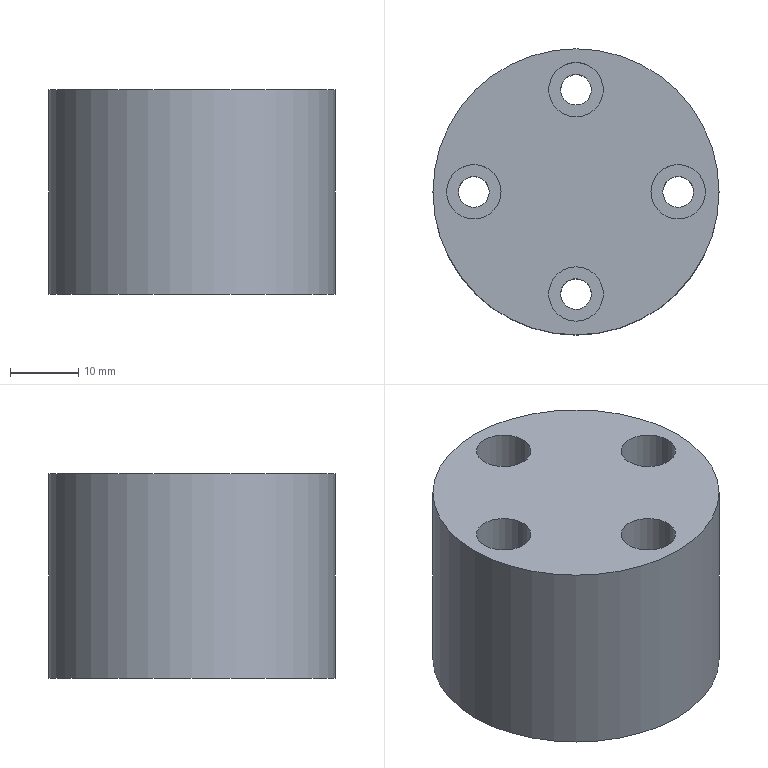NC program | NX | posted with a generic post | part box 42 x 42 x 30 mm
Whole program:
N10 G17 G21 G94 G90
(DRILLING , TOOL : ZXZ)
N12 T01 M6
N14 G54
N16 G17 G0 G90 X0. Y15. S3000 M3
N18 G43 Z30. H1
N20 G94 G81 G98 Z-1. F200. R3.
N22 X-15. Y0.
N24 X0. Y-15.
N26 X15. Y0.
N28 G80
N30 G0 X15. Y0. Z30.
N32 M5
(DRILLING_COPY , TOOL : 4.5ZT)
N34 T02 M6
N36 G54
N38 G17 G0 G90 X0. Y15. S2000 M3
N40 G43 Z30. H2
N42 G94 G83 G98 Z-32.852 F120. Q2. R3.
N44 X-15. Y0.
N46 X0. Y-15.
N48 X15. Y0.
N50 G80
N52 G0 X15. Y0. Z30.
N54 M5
(HOLE_MILLING , TOOL : D6)
N56 T06 M6
N58 G54
N60 G17 G0 G90 X-15. Y0. S4500 M3
N62 G43 Z30. H6
N64 Z0.5
N66 G94 G3 X-14.5 Y-0.5 R0.5 F1400.
N68 X-14. Y0. R0.5
N70 X-14. Y0. Z0.4 I-1. J0.
N72 X-14. Y0. Z0.3 I-1. J0.
N74 X-14. Y0. Z0.2 I-1. J0.
N76 X-14. Y0. Z0.1 I-1. J0.
N78 X-14. Y0. Z0. I-1. J0.
N80 X-14. Y0. Z-0.1 I-1. J0.
N82 X-14. Y0. Z-0.2 I-1. J0.
N84 X-14. Y0. Z-0.3 I-1. J0.
N86 X-14. Y0. Z-0.4 I-1. J0.
N88 X-14. Y0. Z-0.5 I-1. J0.
N90 X-14. Y0. Z-0.6 I-1. J0.
N92 X-14. Y0. Z-0.7 I-1. J0.
N94 X-14. Y0. Z-0.8 I-1. J0.
N96 X-14. Y0. Z-0.9 I-1. J0.
N98 X-14. Y0. Z-1. I-1. J0.
N100 X-14. Y0. Z-1.1 I-1. J0.
N102 X-14. Y0. Z-1.2 I-1. J0.
N104 X-14. Y0. Z-1.3 I-1. J0.
N106 X-14. Y0. Z-1.4 I-1. J0.
N108 X-14. Y0. Z-1.5 I-1. J0.
N110 X-14. Y0. Z-1.6 I-1. J0.
N112 X-14. Y0. Z-1.7 I-1. J0.
N114 X-14. Y0. Z-1.8 I-1. J0.
N116 X-14. Y0. Z-1.9 I-1. J0.
N118 X-14. Y0. Z-2. I-1. J0.
N120 X-14. Y0. Z-2.1 I-1. J0.
N122 X-14. Y0. Z-2.2 I-1. J0.
N124 X-14. Y0. Z-2.3 I-1. J0.
N126 X-14. Y0. Z-2.4 I-1. J0.
N128 X-14. Y0. Z-2.5 I-1. J0.
N130 X-14. Y0. Z-2.6 I-1. J0.
N132 X-14. Y0. Z-2.7 I-1. J0.
N134 X-14. Y0. Z-2.8 I-1. J0.
N136 X-14. Y0. Z-2.9 I-1. J0.
N138 X-14. Y0. Z-3. I-1. J0.
N140 X-14. Y0. Z-3.1 I-1. J0.
N142 X-14. Y0. Z-3.2 I-1. J0.
N144 X-14. Y0. Z-3.3 I-1. J0.
N146 X-14. Y0. Z-3.4 I-1. J0.
N148 X-14. Y0. Z-3.5 I-1. J0.
N150 X-14. Y0. Z-3.6 I-1. J0.
N152 X-14. Y0. Z-3.7 I-1. J0.
N154 X-14. Y0. Z-3.8 I-1. J0.
N156 X-14. Y0. Z-3.9 I-1. J0.
N158 X-14. Y0. Z-4. I-1. J0.
N160 X-14. Y0. Z-4.1 I-1. J0.
N162 X-14. Y0. Z-4.2 I-1. J0.
N164 X-14. Y0. Z-4.3 I-1. J0.
N166 X-14. Y0. Z-4.4 I-1. J0.
N168 X-14. Y0. Z-4.5 I-1. J0.
N170 X-14. Y0. Z-4.6 I-1. J0.
N172 X-14. Y0. Z-4.7 I-1. J0.
N174 X-14. Y0. Z-4.8 I-1. J0.
N176 X-14. Y0. Z-4.9 I-1. J0.
N178 X-14. Y0. Z-5. I-1. J0.
N180 X-14. Y0. Z-5.1 I-1. J0.
N182 X-14. Y0. Z-5.2 I-1. J0.
N184 X-14. Y0. Z-5.3 I-1. J0.
N186 X-14. Y0. Z-5.4 I-1. J0.
N188 X-14. Y0. Z-5.5 I-1. J0.
N190 X-14. Y0. Z-5.6 I-1. J0.
N192 X-14. Y0. Z-5.7 I-1. J0.
N194 X-14. Y0. Z-5.8 I-1. J0.
N196 X-14. Y0. Z-5.9 I-1. J0.
N198 X-14. Y0. Z-6. I-1. J0.
N200 X-15. Y1. R1.
N202 X-14. Y0. R-1.
N204 X-14.5 Y0.5 R0.5
N206 X-15. Y0. R0.5
N208 G0 Z30.
N210 X0. Y15.
N212 Z0.5
N214 G3 X0.5 Y14.5 R0.5
N216 X1. Y15. R0.5
N218 X1. Y15. Z0.4 I-1. J0.
N220 X1. Y15. Z0.3 I-1. J0.
N222 X1. Y15. Z0.2 I-1. J0.
N224 X1. Y15. Z0.1 I-1. J0.
N226 X1. Y15. Z0. I-1. J0.
N228 X1. Y15. Z-0.1 I-1. J0.
N230 X1. Y15. Z-0.2 I-1. J0.
N232 X1. Y15. Z-0.3 I-1. J0.
N234 X1. Y15. Z-0.4 I-1. J0.
N236 X1. Y15. Z-0.5 I-1. J0.
N238 X1. Y15. Z-0.6 I-1. J0.
N240 X1. Y15. Z-0.7 I-1. J0.
N242 X1. Y15. Z-0.8 I-1. J0.
N244 X1. Y15. Z-0.9 I-1. J0.
N246 X1. Y15. Z-1. I-1. J0.
N248 X1. Y15. Z-1.1 I-1. J0.
N250 X1. Y15. Z-1.2 I-1. J0.
N252 X1. Y15. Z-1.3 I-1. J0.
N254 X1. Y15. Z-1.4 I-1. J0.
N256 X1. Y15. Z-1.5 I-1. J0.
N258 X1. Y15. Z-1.6 I-1. J0.
N260 X1. Y15. Z-1.7 I-1. J0.
N262 X1. Y15. Z-1.8 I-1. J0.
N264 X1. Y15. Z-1.9 I-1. J0.
N266 X1. Y15. Z-2. I-1. J0.
N268 X1. Y15. Z-2.1 I-1. J0.
N270 X1. Y15. Z-2.2 I-1. J0.
N272 X1. Y15. Z-2.3 I-1. J0.
N274 X1. Y15. Z-2.4 I-1. J0.
N276 X1. Y15. Z-2.5 I-1. J0.
N278 X1. Y15. Z-2.6 I-1. J0.
N280 X1. Y15. Z-2.7 I-1. J0.
N282 X1. Y15. Z-2.8 I-1. J0.
N284 X1. Y15. Z-2.9 I-1. J0.
N286 X1. Y15. Z-3. I-1. J0.
N288 X1. Y15. Z-3.1 I-1. J0.
N290 X1. Y15. Z-3.2 I-1. J0.
N292 X1. Y15. Z-3.3 I-1. J0.
N294 X1. Y15. Z-3.4 I-1. J0.
N296 X1. Y15. Z-3.5 I-1. J0.
N298 X1. Y15. Z-3.6 I-1. J0.
N300 X1. Y15. Z-3.7 I-1. J0.
N302 X1. Y15. Z-3.8 I-1. J0.
N304 X1. Y15. Z-3.9 I-1. J0.
N306 X1. Y15. Z-4. I-1. J0.
N308 X1. Y15. Z-4.1 I-1. J0.
N310 X1. Y15. Z-4.2 I-1. J0.
N312 X1. Y15. Z-4.3 I-1. J0.
N314 X1. Y15. Z-4.4 I-1. J0.
N316 X1. Y15. Z-4.5 I-1. J0.
N318 X1. Y15. Z-4.6 I-1. J0.
N320 X1. Y15. Z-4.7 I-1. J0.
N322 X1. Y15. Z-4.8 I-1. J0.
N324 X1. Y15. Z-4.9 I-1. J0.
N326 X1. Y15. Z-5. I-1. J0.
N328 X1. Y15. Z-5.1 I-1. J0.
N330 X1. Y15. Z-5.2 I-1. J0.
N332 X1. Y15. Z-5.3 I-1. J0.
N334 X1. Y15. Z-5.4 I-1. J0.
N336 X1. Y15. Z-5.5 I-1. J0.
N338 X1. Y15. Z-5.6 I-1. J0.
N340 X1. Y15. Z-5.7 I-1. J0.
N342 X1. Y15. Z-5.8 I-1. J0.
N344 X1. Y15. Z-5.9 I-1. J0.
N346 X1. Y15. Z-6. I-1. J0.
N348 X0. Y16. R1.
N350 X1. Y15. R-1.
N352 X0.5 Y15.5 R0.5
N354 X0. Y15. R0.5
N356 G0 Z30.
N358 X15. Y0.
N360 Z0.5
N362 G3 X15.5 Y-0.5 R0.5
N364 X16. Y0. R0.5
N366 X16. Y0. Z0.4 I-1. J0.
N368 X16. Y0. Z0.3 I-1. J0.
N370 X16. Y0. Z0.2 I-1. J0.
N372 X16. Y0. Z0.1 I-1. J0.
N374 X16. Y0. Z0. I-1. J0.
N376 X16. Y0. Z-0.1 I-1. J0.
N378 X16. Y0. Z-0.2 I-1. J0.
N380 X16. Y0. Z-0.3 I-1. J0.
N382 X16. Y0. Z-0.4 I-1. J0.
N384 X16. Y0. Z-0.5 I-1. J0.
N386 X16. Y0. Z-0.6 I-1. J0.
N388 X16. Y0. Z-0.7 I-1. J0.
N390 X16. Y0. Z-0.8 I-1. J0.
N392 X16. Y0. Z-0.9 I-1. J0.
N394 X16. Y0. Z-1. I-1. J0.
N396 X16. Y0. Z-1.1 I-1. J0.
N398 X16. Y0. Z-1.2 I-1. J0.
N400 X16. Y0. Z-1.3 I-1. J0.
N402 X16. Y0. Z-1.4 I-1. J0.
N404 X16. Y0. Z-1.5 I-1. J0.
N406 X16. Y0. Z-1.6 I-1. J0.
N408 X16. Y0. Z-1.7 I-1. J0.
N410 X16. Y0. Z-1.8 I-1. J0.
N412 X16. Y0. Z-1.9 I-1. J0.
N414 X16. Y0. Z-2. I-1. J0.
N416 X16. Y0. Z-2.1 I-1. J0.
N418 X16. Y0. Z-2.2 I-1. J0.
N420 X16. Y0. Z-2.3 I-1. J0.
N422 X16. Y0. Z-2.4 I-1. J0.
N424 X16. Y0. Z-2.5 I-1. J0.
N426 X16. Y0. Z-2.6 I-1. J0.
N428 X16. Y0. Z-2.7 I-1. J0.
N430 X16. Y0. Z-2.8 I-1. J0.
N432 X16. Y0. Z-2.9 I-1. J0.
N434 X16. Y0. Z-3. I-1. J0.
N436 X16. Y0. Z-3.1 I-1. J0.
N438 X16. Y0. Z-3.2 I-1. J0.
N440 X16. Y0. Z-3.3 I-1. J0.
N442 X16. Y0. Z-3.4 I-1. J0.
N444 X16. Y0. Z-3.5 I-1. J0.
N446 X16. Y0. Z-3.6 I-1. J0.
N448 X16. Y0. Z-3.7 I-1. J0.
N450 X16. Y0. Z-3.8 I-1. J0.
N452 X16. Y0. Z-3.9 I-1. J0.
N454 X16. Y0. Z-4. I-1. J0.
N456 X16. Y0. Z-4.1 I-1. J0.
N458 X16. Y0. Z-4.2 I-1. J0.
N460 X16. Y0. Z-4.3 I-1. J0.
N462 X16. Y0. Z-4.4 I-1. J0.
N464 X16. Y0. Z-4.5 I-1. J0.
N466 X16. Y0. Z-4.6 I-1. J0.
N468 X16. Y0. Z-4.7 I-1. J0.
N470 X16. Y0. Z-4.8 I-1. J0.
N472 X16. Y0. Z-4.9 I-1. J0.
N474 X16. Y0. Z-5. I-1. J0.
N476 X16. Y0. Z-5.1 I-1. J0.
N478 X16. Y0. Z-5.2 I-1. J0.
N480 X16. Y0. Z-5.3 I-1. J0.
N482 X16. Y0. Z-5.4 I-1. J0.
N484 X16. Y0. Z-5.5 I-1. J0.
N486 X16. Y0. Z-5.6 I-1. J0.
N488 X16. Y0. Z-5.7 I-1. J0.
N490 X16. Y0. Z-5.8 I-1. J0.
N492 X16. Y0. Z-5.9 I-1. J0.
N494 X16. Y0. Z-6. I-1. J0.
N496 X15. Y1. R1.
N498 X16. Y0. R-1.
N500 X15.5 Y0.5 R0.5
N502 X15. Y0. R0.5
N504 G0 Z30.
N506 X0. Y-15.
N508 Z0.5
N510 G3 X0.5 Y-15.5 R0.5
N512 X1. Y-15. R0.5
N514 X1. Y-15. Z0.4 I-1. J0.
N516 X1. Y-15. Z0.3 I-1. J0.
N518 X1. Y-15. Z0.2 I-1. J0.
N520 X1. Y-15. Z0.1 I-1. J0.
N522 X1. Y-15. Z0. I-1. J0.
N524 X1. Y-15. Z-0.1 I-1. J0.
N526 X1. Y-15. Z-0.2 I-1. J0.
N528 X1. Y-15. Z-0.3 I-1. J0.
N530 X1. Y-15. Z-0.4 I-1. J0.
N532 X1. Y-15. Z-0.5 I-1. J0.
N534 X1. Y-15. Z-0.6 I-1. J0.
N536 X1. Y-15. Z-0.7 I-1. J0.
N538 X1. Y-15. Z-0.8 I-1. J0.
N540 X1. Y-15. Z-0.9 I-1. J0.
N542 X1. Y-15. Z-1. I-1. J0.
N544 X1. Y-15. Z-1.1 I-1. J0.
N546 X1. Y-15. Z-1.2 I-1. J0.
N548 X1. Y-15. Z-1.3 I-1. J0.
N550 X1. Y-15. Z-1.4 I-1. J0.
N552 X1. Y-15. Z-1.5 I-1. J0.
N554 X1. Y-15. Z-1.6 I-1. J0.
N556 X1. Y-15. Z-1.7 I-1. J0.
N558 X1. Y-15. Z-1.8 I-1. J0.
N560 X1. Y-15. Z-1.9 I-1. J0.
N562 X1. Y-15. Z-2. I-1. J0.
N564 X1. Y-15. Z-2.1 I-1. J0.
N566 X1. Y-15. Z-2.2 I-1. J0.
N568 X1. Y-15. Z-2.3 I-1. J0.
N570 X1. Y-15. Z-2.4 I-1. J0.
N572 X1. Y-15. Z-2.5 I-1. J0.
N574 X1. Y-15. Z-2.6 I-1. J0.
N576 X1. Y-15. Z-2.7 I-1. J0.
N578 X1. Y-15. Z-2.8 I-1. J0.
N580 X1. Y-15. Z-2.9 I-1. J0.
N582 X1. Y-15. Z-3. I-1. J0.
N584 X1. Y-15. Z-3.1 I-1. J0.
N586 X1. Y-15. Z-3.2 I-1. J0.
N588 X1. Y-15. Z-3.3 I-1. J0.
N590 X1. Y-15. Z-3.4 I-1. J0.
N592 X1. Y-15. Z-3.5 I-1. J0.
N594 X1. Y-15. Z-3.6 I-1. J0.
N596 X1. Y-15. Z-3.7 I-1. J0.
N598 X1. Y-15. Z-3.8 I-1. J0.
N600 X1. Y-15. Z-3.9 I-1. J0.
N602 X1. Y-15. Z-4. I-1. J0.
N604 X1. Y-15. Z-4.1 I-1. J0.
N606 X1. Y-15. Z-4.2 I-1. J0.
N608 X1. Y-15. Z-4.3 I-1. J0.
N610 X1. Y-15. Z-4.4 I-1. J0.
N612 X1. Y-15. Z-4.5 I-1. J0.
N614 X1. Y-15. Z-4.6 I-1. J0.
N616 X1. Y-15. Z-4.7 I-1. J0.
N618 X1. Y-15. Z-4.8 I-1. J0.
N620 X1. Y-15. Z-4.9 I-1. J0.
N622 X1. Y-15. Z-5. I-1. J0.
N624 X1. Y-15. Z-5.1 I-1. J0.
N626 X1. Y-15. Z-5.2 I-1. J0.
N628 X1. Y-15. Z-5.3 I-1. J0.
N630 X1. Y-15. Z-5.4 I-1. J0.
N632 X1. Y-15. Z-5.5 I-1. J0.
N634 X1. Y-15. Z-5.6 I-1. J0.
N636 X1. Y-15. Z-5.7 I-1. J0.
N638 X1. Y-15. Z-5.8 I-1. J0.
N640 X1. Y-15. Z-5.9 I-1. J0.
N642 X1. Y-15. Z-6. I-1. J0.
N644 X0. Y-14. R1.
N646 X1. Y-15. R-1.
N648 X0.5 Y-14.5 R0.5
N650 X0. Y-15. R0.5
N652 G0 Z30.
N654 M5
(ZLEVEL_PROFILE_1_COPY_1 , TOOL : D6A45)
N656 T07 M6
N658 G54
N660 G17 G0 G90 X16.351 Y-1.37 S7500 M3
N662 G43 Z30. H7
N664 Z0.
N666 G94 G1 Z-1. F1000.
N668 X17.824 Y-0.52
N670 G3 X18.124 Y0. R0.6
N672 X15. Y3.124 R3.124
N674 X18.124 Y0. R-3.124
N676 X17.824 Y0.52 R0.6
N678 G1 X16.351 Y1.37
N680 Z0.
N682 G0 Z30.
N684 X-16.351
N686 Z0.
N688 G1 Z-1.
N690 X-17.824 Y0.52
N692 G3 X-18.124 Y0. R0.6
N694 X-15. Y-3.124 R3.124
N696 X-18.124 Y0. R-3.124
N698 X-17.824 Y-0.52 R0.6
N700 G1 X-16.351 Y-1.37
N702 Z0.
N704 G0 Z30.
N706 X1.37 Y16.351
N708 Z0.
N710 G1 Z-1.
N712 X0.52 Y17.824
N714 G3 X0. Y18.124 R0.6
N716 X-3.124 Y15. R3.124
N718 X0. Y18.124 R-3.124
N720 X-0.52 Y17.824 R0.6
N722 G1 X-1.37 Y16.351
N724 Z0.
N726 G0 Z30.
N728 Y-16.351
N730 Z0.
N732 G1 Z-1.
N734 X-0.52 Y-17.824
N736 G3 X0. Y-18.124 R0.6
N738 X3.124 Y-15. R3.124
N740 X0. Y-18.124 R-3.124
N742 X0.52 Y-17.824 R0.6
N744 G1 X1.37 Y-16.351
N746 Z0.
N748 G0 Z30.
N750 M5
N752 M2